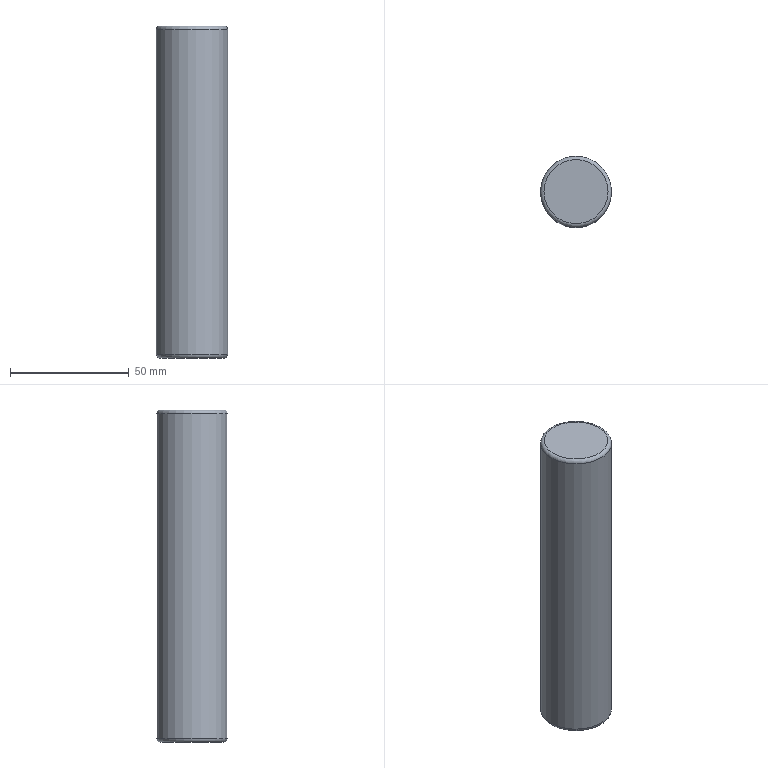Part | STEP file | solid 110 | 1 solid | 5 faces | box 30 x 30 x 140 mm | volume 98871 mm3 | plane 2 | torus 2 | cylinder 1 | commonest cylinder face diameters 30 x1